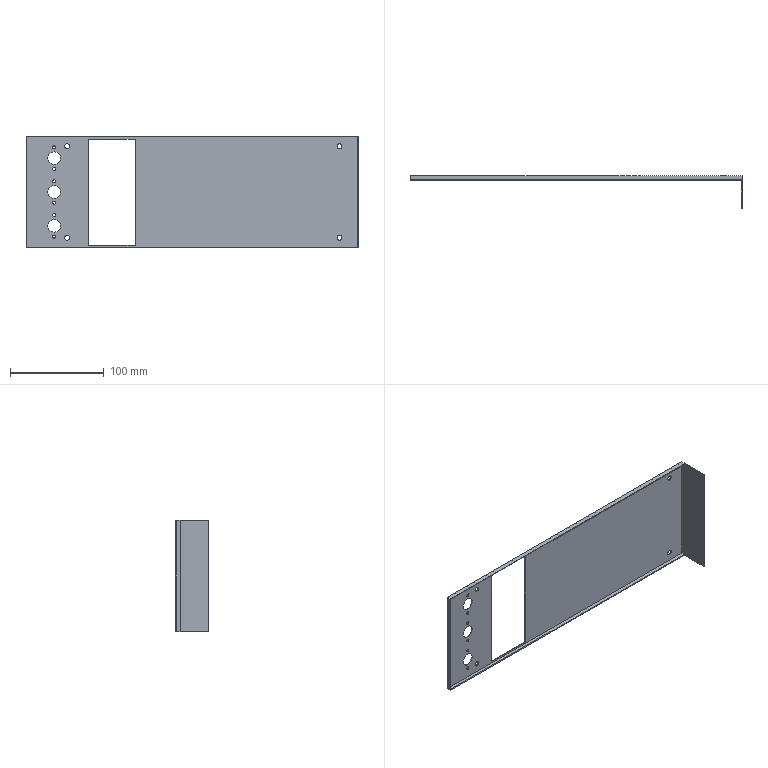Part | SolidWorks | features MoveFace 15, ICE 6, Cut 1, Extrusion 1 | 1 solid | 42 faces | box 353.4 x 34.5 x 119.15 mm | volume 42763 mm3 | cylinder 26 | plane 16 | commonest cylinder face diameters 3.2 x12 5.2 x8 13.5 x6
STEP:
#1=CARTESIAN_POINT('',(-211.2,0.5,49.1));
#2=VERTEX_POINT('',#1);
#3=CARTESIAN_POINT('',(-211.2,0.5,45.9));
#4=VERTEX_POINT('',#3);
#5=CARTESIAN_POINT('',(-211.2,0.5,47.5));
#6=DIRECTION('',(0.,-1.,0.));
#7=DIRECTION('',(0.,0.,-1.));
#8=AXIS2_PLACEMENT_3D('',#5,#6,#7);
#9=CIRCLE('',#8,1.6);
#10=EDGE_CURVE('',#2,#4,#9,.T.);
#11=ORIENTED_EDGE('',*,*,#10,.T.);
#12=CARTESIAN_POINT('',(-211.2,1.5,45.9));
#13=VERTEX_POINT('',#12);
#14=CARTESIAN_POINT('',(-211.2,-3.,45.9));
#15=DIRECTION('',(0.,1.,0.));
#16=VECTOR('',#15,1000.);
#17=LINE('',#14,#16);
#18=EDGE_CURVE('',#4,#13,#17,.T.);
#19=ORIENTED_EDGE('',*,*,#18,.T.);
#20=CARTESIAN_POINT('',(-211.2,1.5,49.1));
#21=VERTEX_POINT('',#20);
#22=CARTESIAN_POINT('',(-211.2,1.5,47.5));
#23=DIRECTION('',(0.,1.,0.));
#24=DIRECTION('',(0.,0.,1.));
#25=AXIS2_PLACEMENT_3D('',#22,#23,#24);
#26=CIRCLE('',#25,1.6);
#27=EDGE_CURVE('',#13,#21,#26,.T.);
#28=ORIENTED_EDGE('',*,*,#27,.T.);
#29=CARTESIAN_POINT('',(-211.2,-3.,49.1));
#30=DIRECTION('',(0.,1.,0.));
#31=VECTOR('',#30,1000.);
#32=LINE('',#29,#31);
#33=EDGE_CURVE('',#2,#21,#32,.T.);
#34=ORIENTED_EDGE('',*,*,#33,.F.);
#35=EDGE_LOOP('',(#11,#19,#28,#34));
#36=FACE_OUTER_BOUND('',#35,.T.);
#37=CARTESIAN_POINT('',(-211.2,-3.,47.5));
#38=DIRECTION('',(0.,1.,0.));
#39=DIRECTION('',(0.,0.,1.));
#40=AXIS2_PLACEMENT_3D('',#37,#38,#39);
#41=CYLINDRICAL_SURFACE('',#40,1.6);
#42=ADVANCED_FACE('',(#36),#41,.F.);
#43=CARTESIAN_POINT('',(-211.2,0.5,26.1));
#44=VERTEX_POINT('',#43);
#45=CARTESIAN_POINT('',(-211.2,0.5,22.9));
#46=VERTEX_POINT('',#45);
#47=CARTESIAN_POINT('',(-211.2,0.5,24.5));
#48=DIRECTION('',(0.,-1.,0.));
#49=DIRECTION('',(0.,0.,-1.));
#50=AXIS2_PLACEMENT_3D('',#47,#48,#49);
#51=CIRCLE('',#50,1.6);
#52=EDGE_CURVE('',#44,#46,#51,.T.);
#53=ORIENTED_EDGE('',*,*,#52,.T.);
#54=CARTESIAN_POINT('',(-211.2,1.5,22.9));
#55=VERTEX_POINT('',#54);
#56=CARTESIAN_POINT('',(-211.2,-3.,22.9));
#57=DIRECTION('',(0.,1.,0.));
#58=VECTOR('',#57,1000.);
#59=LINE('',#56,#58);
#60=EDGE_CURVE('',#46,#55,#59,.T.);
#61=ORIENTED_EDGE('',*,*,#60,.T.);
#62=CARTESIAN_POINT('',(-211.2,1.5,26.1));
#63=VERTEX_POINT('',#62);
#64=CARTESIAN_POINT('',(-211.2,1.5,24.5));
#65=DIRECTION('',(0.,1.,0.));
#66=DIRECTION('',(0.,0.,1.));
#67=AXIS2_PLACEMENT_3D('',#64,#65,#66);
#68=CIRCLE('',#67,1.6);
#69=EDGE_CURVE('',#55,#63,#68,.T.);
#70=ORIENTED_EDGE('',*,*,#69,.T.);
#71=CARTESIAN_POINT('',(-211.2,-3.,26.1));
#72=DIRECTION('',(0.,1.,0.));
#73=VECTOR('',#72,1000.);
#74=LINE('',#71,#73);
#75=EDGE_CURVE('',#44,#63,#74,.T.);
#76=ORIENTED_EDGE('',*,*,#75,.F.);
#77=EDGE_LOOP('',(#53,#61,#70,#76));
#78=FACE_OUTER_BOUND('',#77,.T.);
#79=CARTESIAN_POINT('',(-211.2,-3.,24.5));
#80=DIRECTION('',(0.,1.,0.));
#81=DIRECTION('',(0.,0.,1.));
#82=AXIS2_PLACEMENT_3D('',#79,#80,#81);
#83=CYLINDRICAL_SURFACE('',#82,1.6);
#84=ADVANCED_FACE('',(#78),#83,.F.);
#85=CARTESIAN_POINT('',(-211.2,0.5,13.1));
#86=VERTEX_POINT('',#85);
#87=CARTESIAN_POINT('',(-211.2,0.5,9.9));
#88=VERTEX_POINT('',#87);
#89=CARTESIAN_POINT('',(-211.2,0.5,11.5));
#90=DIRECTION('',(0.,-1.,0.));
#91=DIRECTION('',(0.,0.,-1.));
#92=AXIS2_PLACEMENT_3D('',#89,#90,#91);
#93=CIRCLE('',#92,1.6);
#94=EDGE_CURVE('',#86,#88,#93,.T.);
#95=ORIENTED_EDGE('',*,*,#94,.T.);
#96=CARTESIAN_POINT('',(-211.2,1.5,9.9));
#97=VERTEX_POINT('',#96);
#98=CARTESIAN_POINT('',(-211.2,-3.,9.9));
#99=DIRECTION('',(0.,1.,0.));
#100=VECTOR('',#99,1000.);
#101=LINE('',#98,#100);
#102=EDGE_CURVE('',#88,#97,#101,.T.);
#103=ORIENTED_EDGE('',*,*,#102,.T.);
#104=CARTESIAN_POINT('',(-211.2,1.5,13.1));
#105=VERTEX_POINT('',#104);
#106=CARTESIAN_POINT('',(-211.2,1.5,11.5));
#107=DIRECTION('',(0.,1.,0.));
#108=DIRECTION('',(0.,0.,1.));
#109=AXIS2_PLACEMENT_3D('',#106,#107,#108);
#110=CIRCLE('',#109,1.6);
#111=EDGE_CURVE('',#97,#105,#110,.T.);
#112=ORIENTED_EDGE('',*,*,#111,.T.);
#113=CARTESIAN_POINT('',(-211.2,-3.,13.1));
#114=DIRECTION('',(0.,1.,0.));
#115=VECTOR('',#114,1000.);
#116=LINE('',#113,#115);
#117=EDGE_CURVE('',#86,#105,#116,.T.);
#118=ORIENTED_EDGE('',*,*,#117,.F.);
#119=EDGE_LOOP('',(#95,#103,#112,#118));
#120=FACE_OUTER_BOUND('',#119,.T.);
#121=CARTESIAN_POINT('',(-211.2,-3.,11.5));
#122=DIRECTION('',(0.,1.,0.));
#123=DIRECTION('',(0.,0.,1.));
#124=AXIS2_PLACEMENT_3D('',#121,#122,#123);
#125=CYLINDRICAL_SURFACE('',#124,1.6);
#126=ADVANCED_FACE('',(#120),#125,.F.);
#127=CARTESIAN_POINT('',(-211.2,0.5,-9.9));
#128=VERTEX_POINT('',#127);
#129=CARTESIAN_POINT('',(-211.2,0.5,-13.1));
#130=VERTEX_POINT('',#129);
#131=CARTESIAN_POINT('',(-211.2,0.5,-11.5));
#132=DIRECTION('',(0.,-1.,0.));
#133=DIRECTION('',(0.,0.,-1.));
#134=AXIS2_PLACEMENT_3D('',#131,#132,#133);
#135=CIRCLE('',#134,1.6);
#136=EDGE_CURVE('',#128,#130,#135,.T.);
#137=ORIENTED_EDGE('',*,*,#136,.T.);
#138=CARTESIAN_POINT('',(-211.2,1.5,-13.1));
#139=VERTEX_POINT('',#138);
#140=CARTESIAN_POINT('',(-211.2,-3.,-13.1));
#141=DIRECTION('',(0.,1.,0.));
#142=VECTOR('',#141,1000.);
#143=LINE('',#140,#142);
#144=EDGE_CURVE('',#130,#139,#143,.T.);
#145=ORIENTED_EDGE('',*,*,#144,.T.);
#146=CARTESIAN_POINT('',(-211.2,1.5,-9.9));
#147=VERTEX_POINT('',#146);
#148=CARTESIAN_POINT('',(-211.2,1.5,-11.5));
#149=DIRECTION('',(0.,1.,0.));
#150=DIRECTION('',(0.,0.,1.));
#151=AXIS2_PLACEMENT_3D('',#148,#149,#150);
#152=CIRCLE('',#151,1.6);
#153=EDGE_CURVE('',#139,#147,#152,.T.);
#154=ORIENTED_EDGE('',*,*,#153,.T.);
#155=CARTESIAN_POINT('',(-211.2,-3.,-9.9));
#156=DIRECTION('',(0.,1.,0.));
#157=VECTOR('',#156,1000.);
#158=LINE('',#155,#157);
#159=EDGE_CURVE('',#128,#147,#158,.T.);
#160=ORIENTED_EDGE('',*,*,#159,.F.);
#161=EDGE_LOOP('',(#137,#145,#154,#160));
#162=FACE_OUTER_BOUND('',#161,.T.);
#163=CARTESIAN_POINT('',(-211.2,-3.,-11.5));
#164=DIRECTION('',(0.,1.,0.));
#165=DIRECTION('',(0.,0.,1.));
#166=AXIS2_PLACEMENT_3D('',#163,#164,#165);
#167=CYLINDRICAL_SURFACE('',#166,1.6);
#168=ADVANCED_FACE('',(#162),#167,.F.);
#169=CARTESIAN_POINT('',(-211.2,0.5,-22.9));
#170=VERTEX_POINT('',#169);
#171=CARTESIAN_POINT('',(-211.2,0.5,-26.1));
#172=VERTEX_POINT('',#171);
#173=CARTESIAN_POINT('',(-211.2,0.5,-24.5));
#174=DIRECTION('',(0.,-1.,0.));
#175=DIRECTION('',(0.,0.,-1.));
#176=AXIS2_PLACEMENT_3D('',#173,#174,#175);
#177=CIRCLE('',#176,1.6);
#178=EDGE_CURVE('',#170,#172,#177,.T.);
#179=ORIENTED_EDGE('',*,*,#178,.T.);
#180=CARTESIAN_POINT('',(-211.2,1.5,-26.1));
#181=VERTEX_POINT('',#180);
#182=CARTESIAN_POINT('',(-211.2,-3.,-26.1));
#183=DIRECTION('',(0.,1.,0.));
#184=VECTOR('',#183,1000.);
#185=LINE('',#182,#184);
#186=EDGE_CURVE('',#172,#181,#185,.T.);
#187=ORIENTED_EDGE('',*,*,#186,.T.);
#188=CARTESIAN_POINT('',(-211.2,1.5,-22.9));
#189=VERTEX_POINT('',#188);
#190=CARTESIAN_POINT('',(-211.2,1.5,-24.5));
#191=DIRECTION('',(0.,1.,0.));
#192=DIRECTION('',(0.,0.,1.));
#193=AXIS2_PLACEMENT_3D('',#190,#191,#192);
#194=CIRCLE('',#193,1.6);
#195=EDGE_CURVE('',#181,#189,#194,.T.);
#196=ORIENTED_EDGE('',*,*,#195,.T.);
#197=CARTESIAN_POINT('',(-211.2,-3.,-22.9));
#198=DIRECTION('',(0.,1.,0.));
#199=VECTOR('',#198,1000.);
#200=LINE('',#197,#199);
#201=EDGE_CURVE('',#170,#189,#200,.T.);
#202=ORIENTED_EDGE('',*,*,#201,.F.);
#203=EDGE_LOOP('',(#179,#187,#196,#202));
#204=FACE_OUTER_BOUND('',#203,.T.);
#205=CARTESIAN_POINT('',(-211.2,-3.,-24.5));
#206=DIRECTION('',(0.,1.,0.));
#207=DIRECTION('',(0.,0.,1.));
#208=AXIS2_PLACEMENT_3D('',#205,#206,#207);
#209=CYLINDRICAL_SURFACE('',#208,1.6);
#210=ADVANCED_FACE('',(#204),#209,.F.);
#211=CARTESIAN_POINT('',(-211.2,0.5,-45.9));
#212=VERTEX_POINT('',#211);
#213=CARTESIAN_POINT('',(-211.2,0.5,-49.1));
#214=VERTEX_POINT('',#213);
#215=CARTESIAN_POINT('',(-211.2,0.5,-47.5));
#216=DIRECTION('',(0.,-1.,0.));
#217=DIRECTION('',(0.,0.,-1.));
#218=AXIS2_PLACEMENT_3D('',#215,#216,#217);
#219=CIRCLE('',#218,1.6);
#220=EDGE_CURVE('',#212,#214,#219,.T.);
#221=ORIENTED_EDGE('',*,*,#220,.T.);
#222=CARTESIAN_POINT('',(-211.2,1.5,-49.1));
#223=VERTEX_POINT('',#222);
#224=CARTESIAN_POINT('',(-211.2,-3.,-49.1));
#225=DIRECTION('',(0.,1.,0.));
#226=VECTOR('',#225,1000.);
#227=LINE('',#224,#226);
#228=EDGE_CURVE('',#214,#223,#227,.T.);
#229=ORIENTED_EDGE('',*,*,#228,.T.);
#230=CARTESIAN_POINT('',(-211.2,1.5,-45.9));
#231=VERTEX_POINT('',#230);
#232=CARTESIAN_POINT('',(-211.2,1.5,-47.5));
#233=DIRECTION('',(0.,1.,0.));
#234=DIRECTION('',(0.,0.,1.));
#235=AXIS2_PLACEMENT_3D('',#232,#233,#234);
#236=CIRCLE('',#235,1.6);
#237=EDGE_CURVE('',#223,#231,#236,.T.);
#238=ORIENTED_EDGE('',*,*,#237,.T.);
#239=CARTESIAN_POINT('',(-211.2,-3.,-45.9));
#240=DIRECTION('',(0.,1.,0.));
#241=VECTOR('',#240,1000.);
#242=LINE('',#239,#241);
#243=EDGE_CURVE('',#212,#231,#242,.T.);
#244=ORIENTED_EDGE('',*,*,#243,.F.);
#245=EDGE_LOOP('',(#221,#229,#238,#244));
#246=FACE_OUTER_BOUND('',#245,.T.);
#247=CARTESIAN_POINT('',(-211.2,-3.,-47.5));
#248=DIRECTION('',(0.,1.,0.));
#249=DIRECTION('',(0.,0.,1.));
#250=AXIS2_PLACEMENT_3D('',#247,#248,#249);
#251=CYLINDRICAL_SURFACE('',#250,1.6);
#252=ADVANCED_FACE('',(#246),#251,.F.);
#253=CARTESIAN_POINT('',(-211.2,0.5,42.75));
#254=VERTEX_POINT('',#253);
#255=CARTESIAN_POINT('',(-211.2,0.5,29.25));
#256=VERTEX_POINT('',#255);
#257=CARTESIAN_POINT('',(-211.2,0.5,36.));
#258=DIRECTION('',(0.,-1.,0.));
#259=DIRECTION('',(0.,0.,-1.));
#260=AXIS2_PLACEMENT_3D('',#257,#258,#259);
#261=CIRCLE('',#260,6.75);
#262=EDGE_CURVE('',#254,#256,#261,.T.);
#263=ORIENTED_EDGE('',*,*,#262,.T.);
#264=CARTESIAN_POINT('',(-211.2,1.5,29.25));
#265=VERTEX_POINT('',#264);
#266=CARTESIAN_POINT('',(-211.2,-8.5,29.25));
#267=DIRECTION('',(0.,1.,0.));
#268=VECTOR('',#267,1000.);
#269=LINE('',#266,#268);
#270=EDGE_CURVE('',#256,#265,#269,.T.);
#271=ORIENTED_EDGE('',*,*,#270,.T.);
#272=CARTESIAN_POINT('',(-211.2,1.5,42.75));
#273=VERTEX_POINT('',#272);
#274=CARTESIAN_POINT('',(-211.2,1.5,36.));
#275=DIRECTION('',(0.,1.,0.));
#276=DIRECTION('',(0.,0.,1.));
#277=AXIS2_PLACEMENT_3D('',#274,#275,#276);
#278=CIRCLE('',#277,6.75);
#279=EDGE_CURVE('',#265,#273,#278,.T.);
#280=ORIENTED_EDGE('',*,*,#279,.T.);
#281=CARTESIAN_POINT('',(-211.2,-8.5,42.75));
#282=DIRECTION('',(0.,1.,0.));
#283=VECTOR('',#282,1000.);
#284=LINE('',#281,#283);
#285=EDGE_CURVE('',#254,#273,#284,.T.);
#286=ORIENTED_EDGE('',*,*,#285,.F.);
#287=EDGE_LOOP('',(#263,#271,#280,#286));
#288=FACE_OUTER_BOUND('',#287,.T.);
#289=CARTESIAN_POINT('',(-211.2,-8.5,36.));
#290=DIRECTION('',(0.,1.,0.));
#291=DIRECTION('',(0.,0.,1.));
#292=AXIS2_PLACEMENT_3D('',#289,#290,#291);
#293=CYLINDRICAL_SURFACE('',#292,6.75);
#294=ADVANCED_FACE('',(#288),#293,.F.);
#295=CARTESIAN_POINT('',(-211.2,0.5,6.75));
#296=VERTEX_POINT('',#295);
#297=CARTESIAN_POINT('',(-211.2,0.5,-6.75));
#298=VERTEX_POINT('',#297);
#299=CARTESIAN_POINT('',(-211.2,0.5,0.));
#300=DIRECTION('',(0.,-1.,0.));
#301=DIRECTION('',(0.,0.,-1.));
#302=AXIS2_PLACEMENT_3D('',#299,#300,#301);
#303=CIRCLE('',#302,6.75);
#304=EDGE_CURVE('',#296,#298,#303,.T.);
#305=ORIENTED_EDGE('',*,*,#304,.T.);
#306=CARTESIAN_POINT('',(-211.2,1.5,-6.75));
#307=VERTEX_POINT('',#306);
#308=CARTESIAN_POINT('',(-211.2,-8.5,-6.75));
#309=DIRECTION('',(0.,1.,0.));
#310=VECTOR('',#309,1000.);
#311=LINE('',#308,#310);
#312=EDGE_CURVE('',#298,#307,#311,.T.);
#313=ORIENTED_EDGE('',*,*,#312,.T.);
#314=CARTESIAN_POINT('',(-211.2,1.5,6.75));
#315=VERTEX_POINT('',#314);
#316=CARTESIAN_POINT('',(-211.2,1.5,0.));
#317=DIRECTION('',(0.,1.,0.));
#318=DIRECTION('',(0.,0.,1.));
#319=AXIS2_PLACEMENT_3D('',#316,#317,#318);
#320=CIRCLE('',#319,6.75);
#321=EDGE_CURVE('',#307,#315,#320,.T.);
#322=ORIENTED_EDGE('',*,*,#321,.T.);
#323=CARTESIAN_POINT('',(-211.2,-8.5,6.75));
#324=DIRECTION('',(0.,1.,0.));
#325=VECTOR('',#324,1000.);
#326=LINE('',#323,#325);
#327=EDGE_CURVE('',#296,#315,#326,.T.);
#328=ORIENTED_EDGE('',*,*,#327,.F.);
#329=EDGE_LOOP('',(#305,#313,#322,#328));
#330=FACE_OUTER_BOUND('',#329,.T.);
#331=CARTESIAN_POINT('',(-211.2,-8.5,0.));
#332=DIRECTION('',(0.,1.,0.));
#333=DIRECTION('',(0.,0.,1.));
#334=AXIS2_PLACEMENT_3D('',#331,#332,#333);
#335=CYLINDRICAL_SURFACE('',#334,6.75);
#336=ADVANCED_FACE('',(#330),#335,.F.);
#337=CARTESIAN_POINT('',(-211.2,0.5,-29.25));
#338=VERTEX_POINT('',#337);
#339=CARTESIAN_POINT('',(-211.2,0.5,-42.75));
#340=VERTEX_POINT('',#339);
#341=CARTESIAN_POINT('',(-211.2,0.5,-36.));
#342=DIRECTION('',(0.,-1.,0.));
#343=DIRECTION('',(0.,0.,-1.));
#344=AXIS2_PLACEMENT_3D('',#341,#342,#343);
#345=CIRCLE('',#344,6.75);
#346=EDGE_CURVE('',#338,#340,#345,.T.);
#347=ORIENTED_EDGE('',*,*,#346,.T.);
#348=CARTESIAN_POINT('',(-211.2,1.5,-42.75));
#349=VERTEX_POINT('',#348);
#350=CARTESIAN_POINT('',(-211.2,-8.5,-42.75));
#351=DIRECTION('',(0.,1.,0.));
#352=VECTOR('',#351,1000.);
#353=LINE('',#350,#352);
#354=EDGE_CURVE('',#340,#349,#353,.T.);
#355=ORIENTED_EDGE('',*,*,#354,.T.);
#356=CARTESIAN_POINT('',(-211.2,1.5,-29.25));
#357=VERTEX_POINT('',#356);
#358=CARTESIAN_POINT('',(-211.2,1.5,-36.));
#359=DIRECTION('',(0.,1.,0.));
#360=DIRECTION('',(0.,0.,1.));
#361=AXIS2_PLACEMENT_3D('',#358,#359,#360);
#362=CIRCLE('',#361,6.75);
#363=EDGE_CURVE('',#349,#357,#362,.T.);
#364=ORIENTED_EDGE('',*,*,#363,.T.);
#365=CARTESIAN_POINT('',(-211.2,-8.5,-29.25));
#366=DIRECTION('',(0.,1.,0.));
#367=VECTOR('',#366,1000.);
#368=LINE('',#365,#367);
#369=EDGE_CURVE('',#338,#357,#368,.T.);
#370=ORIENTED_EDGE('',*,*,#369,.F.);
#371=EDGE_LOOP('',(#347,#355,#364,#370));
#372=FACE_OUTER_BOUND('',#371,.T.);
#373=CARTESIAN_POINT('',(-211.2,-8.5,-36.));
#374=DIRECTION('',(0.,1.,0.));
#375=DIRECTION('',(0.,0.,1.));
#376=AXIS2_PLACEMENT_3D('',#373,#374,#375);
#377=CYLINDRICAL_SURFACE('',#376,6.75);
#378=ADVANCED_FACE('',(#372),#377,.F.);
#379=CARTESIAN_POINT('',(92.5,0.5,-46.025));
#380=VERTEX_POINT('',#379);
#381=CARTESIAN_POINT('',(92.5,0.5,-51.225));
#382=VERTEX_POINT('',#381);
#383=CARTESIAN_POINT('',(92.5,0.5,-48.625));
#384=DIRECTION('',(0.,-1.,0.));
#385=DIRECTION('',(0.,0.,-1.));
#386=AXIS2_PLACEMENT_3D('',#383,#384,#385);
#387=CIRCLE('',#386,2.6);
#388=EDGE_CURVE('',#380,#382,#387,.T.);
#389=ORIENTED_EDGE('',*,*,#388,.T.);
#390=CARTESIAN_POINT('',(92.5,1.5,-51.225));
#391=VERTEX_POINT('',#390);
#392=CARTESIAN_POINT('',(92.5,-330.5,-51.225));
#393=DIRECTION('',(0.,1.,0.));
#394=VECTOR('',#393,1000.);
#395=LINE('',#392,#394);
#396=EDGE_CURVE('',#382,#391,#395,.T.);
#397=ORIENTED_EDGE('',*,*,#396,.T.);
#398=CARTESIAN_POINT('',(92.5,1.5,-46.025));
#399=VERTEX_POINT('',#398);
#400=CARTESIAN_POINT('',(92.5,1.5,-48.625));
#401=DIRECTION('',(0.,1.,0.));
#402=DIRECTION('',(0.,0.,1.));
#403=AXIS2_PLACEMENT_3D('',#400,#401,#402);
#404=CIRCLE('',#403,2.6);
#405=EDGE_CURVE('',#391,#399,#404,.T.);
#406=ORIENTED_EDGE('',*,*,#405,.T.);
#407=CARTESIAN_POINT('',(92.5,-330.5,-46.025));
#408=DIRECTION('',(0.,1.,0.));
#409=VECTOR('',#408,1000.);
#410=LINE('',#407,#409);
#411=EDGE_CURVE('',#380,#399,#410,.T.);
#412=ORIENTED_EDGE('',*,*,#411,.F.);
#413=EDGE_LOOP('',(#389,#397,#406,#412));
#414=FACE_OUTER_BOUND('',#413,.T.);
#415=CARTESIAN_POINT('',(92.5,-330.5,-48.625));
#416=DIRECTION('',(0.,1.,0.));
#417=DIRECTION('',(0.,0.,1.));
#418=AXIS2_PLACEMENT_3D('',#415,#416,#417);
#419=CYLINDRICAL_SURFACE('',#418,2.6);
#420=ADVANCED_FACE('',(#414),#419,.F.);
#421=CARTESIAN_POINT('',(-197.5,0.5,51.225));
#422=VERTEX_POINT('',#421);
#423=CARTESIAN_POINT('',(-197.5,0.5,46.025));
#424=VERTEX_POINT('',#423);
#425=CARTESIAN_POINT('',(-197.5,0.5,48.625));
#426=DIRECTION('',(0.,-1.,0.));
#427=DIRECTION('',(0.,0.,-1.));
#428=AXIS2_PLACEMENT_3D('',#425,#426,#427);
#429=CIRCLE('',#428,2.6);
#430=EDGE_CURVE('',#422,#424,#429,.T.);
#431=ORIENTED_EDGE('',*,*,#430,.T.);
#432=CARTESIAN_POINT('',(-197.5,1.5,46.025));
#433=VERTEX_POINT('',#432);
#434=CARTESIAN_POINT('',(-197.5,-330.5,46.025));
#435=DIRECTION('',(0.,1.,0.));
#436=VECTOR('',#435,1000.);
#437=LINE('',#434,#436);
#438=EDGE_CURVE('',#424,#433,#437,.T.);
#439=ORIENTED_EDGE('',*,*,#438,.T.);
#440=CARTESIAN_POINT('',(-197.5,1.5,51.225));
#441=VERTEX_POINT('',#440);
#442=CARTESIAN_POINT('',(-197.5,1.5,48.625));
#443=DIRECTION('',(0.,1.,0.));
#444=DIRECTION('',(0.,0.,1.));
#445=AXIS2_PLACEMENT_3D('',#442,#443,#444);
#446=CIRCLE('',#445,2.6);
#447=EDGE_CURVE('',#433,#441,#446,.T.);
#448=ORIENTED_EDGE('',*,*,#447,.T.);
#449=CARTESIAN_POINT('',(-197.5,-330.5,51.225));
#450=DIRECTION('',(0.,1.,0.));
#451=VECTOR('',#450,1000.);
#452=LINE('',#449,#451);
#453=EDGE_CURVE('',#422,#441,#452,.T.);
#454=ORIENTED_EDGE('',*,*,#453,.F.);
#455=EDGE_LOOP('',(#431,#439,#448,#454));
#456=FACE_OUTER_BOUND('',#455,.T.);
#457=CARTESIAN_POINT('',(-197.5,-330.5,48.625));
#458=DIRECTION('',(0.,1.,0.));
#459=DIRECTION('',(0.,0.,1.));
#460=AXIS2_PLACEMENT_3D('',#457,#458,#459);
#461=CYLINDRICAL_SURFACE('',#460,2.6);
#462=ADVANCED_FACE('',(#456),#461,.F.);
#463=CARTESIAN_POINT('',(-197.5,0.5,-46.025));
#464=VERTEX_POINT('',#463);
#465=CARTESIAN_POINT('',(-197.5,0.5,-51.225));
#466=VERTEX_POINT('',#465);
#467=CARTESIAN_POINT('',(-197.5,0.5,-48.625));
#468=DIRECTION('',(0.,-1.,0.));
#469=DIRECTION('',(0.,0.,-1.));
#470=AXIS2_PLACEMENT_3D('',#467,#468,#469);
#471=CIRCLE('',#470,2.6);
#472=EDGE_CURVE('',#464,#466,#471,.T.);
#473=ORIENTED_EDGE('',*,*,#472,.T.);
#474=CARTESIAN_POINT('',(-197.5,1.5,-51.225));
#475=VERTEX_POINT('',#474);
#476=CARTESIAN_POINT('',(-197.5,-330.5,-51.225));
#477=DIRECTION('',(0.,1.,0.));
#478=VECTOR('',#477,1000.);
#479=LINE('',#476,#478);
#480=EDGE_CURVE('',#466,#475,#479,.T.);
#481=ORIENTED_EDGE('',*,*,#480,.T.);
#482=CARTESIAN_POINT('',(-197.5,1.5,-46.025));
#483=VERTEX_POINT('',#482);
#484=CARTESIAN_POINT('',(-197.5,1.5,-48.625));
#485=DIRECTION('',(0.,1.,0.));
#486=DIRECTION('',(0.,0.,1.));
#487=AXIS2_PLACEMENT_3D('',#484,#485,#486);
#488=CIRCLE('',#487,2.6);
#489=EDGE_CURVE('',#475,#483,#488,.T.);
#490=ORIENTED_EDGE('',*,*,#489,.T.);
#491=CARTESIAN_POINT('',(-197.5,-330.5,-46.025));
#492=DIRECTION('',(0.,1.,0.));
#493=VECTOR('',#492,1000.);
#494=LINE('',#491,#493);
#495=EDGE_CURVE('',#464,#483,#494,.T.);
#496=ORIENTED_EDGE('',*,*,#495,.F.);
#497=EDGE_LOOP('',(#473,#481,#490,#496));
#498=FACE_OUTER_BOUND('',#497,.T.);
#499=CARTESIAN_POINT('',(-197.5,-330.5,-48.625));
#500=DIRECTION('',(0.,1.,0.));
#501=DIRECTION('',(0.,0.,1.));
#502=AXIS2_PLACEMENT_3D('',#499,#500,#501);
#503=CYLINDRICAL_SURFACE('',#502,2.6);
#504=ADVANCED_FACE('',(#498),#503,.F.);
#505=CARTESIAN_POINT('',(92.5,0.5,51.225));
#506=VERTEX_POINT('',#505);
#507=CARTESIAN_POINT('',(92.5,0.5,46.025));
#508=VERTEX_POINT('',#507);
#509=CARTESIAN_POINT('',(92.5,0.5,48.625));
#510=DIRECTION('',(0.,-1.,0.));
#511=DIRECTION('',(0.,0.,-1.));
#512=AXIS2_PLACEMENT_3D('',#509,#510,#511);
#513=CIRCLE('',#512,2.6);
#514=EDGE_CURVE('',#506,#508,#513,.T.);
#515=ORIENTED_EDGE('',*,*,#514,.T.);
#516=CARTESIAN_POINT('',(92.5,1.5,46.025));
#517=VERTEX_POINT('',#516);
#518=CARTESIAN_POINT('',(92.5,-330.5,46.025));
#519=DIRECTION('',(0.,1.,0.));
#520=VECTOR('',#519,1000.);
#521=LINE('',#518,#520);
#522=EDGE_CURVE('',#508,#517,#521,.T.);
#523=ORIENTED_EDGE('',*,*,#522,.T.);
#524=CARTESIAN_POINT('',(92.5,1.5,51.225));
#525=VERTEX_POINT('',#524);
#526=CARTESIAN_POINT('',(92.5,1.5,48.625));
#527=DIRECTION('',(0.,1.,0.));
#528=DIRECTION('',(0.,0.,1.));
#529=AXIS2_PLACEMENT_3D('',#526,#527,#528);
#530=CIRCLE('',#529,2.6);
#531=EDGE_CURVE('',#517,#525,#530,.T.);
#532=ORIENTED_EDGE('',*,*,#531,.T.);
#533=CARTESIAN_POINT('',(92.5,-330.5,51.225));
#534=DIRECTION('',(0.,1.,0.));
#535=VECTOR('',#534,1000.);
#536=LINE('',#533,#535);
#537=EDGE_CURVE('',#506,#525,#536,.T.);
#538=ORIENTED_EDGE('',*,*,#537,.F.);
#539=EDGE_LOOP('',(#515,#523,#532,#538));
#540=FACE_OUTER_BOUND('',#539,.T.);
#541=CARTESIAN_POINT('',(92.5,-330.5,48.625));
#542=DIRECTION('',(0.,1.,0.));
#543=DIRECTION('',(0.,0.,1.));
#544=AXIS2_PLACEMENT_3D('',#541,#542,#543);
#545=CYLINDRICAL_SURFACE('',#544,2.6);
#546=ADVANCED_FACE('',(#540),#545,.F.);
#547=CARTESIAN_POINT('',(-211.2,1.5,47.5));
#548=DIRECTION('',(0.,1.,0.));
#549=DIRECTION('',(0.,0.,1.));
#550=AXIS2_PLACEMENT_3D('',#547,#548,#549);
#551=CIRCLE('',#550,1.6);
#552=EDGE_CURVE('',#21,#13,#551,.T.);
#553=ORIENTED_EDGE('',*,*,#552,.F.);
#554=ORIENTED_EDGE('',*,*,#27,.F.);
#555=EDGE_LOOP('',(#553,#554));
#556=FACE_BOUND('',#555,.T.);
#557=CARTESIAN_POINT('',(-211.2,1.5,24.5));
#558=DIRECTION('',(0.,1.,0.));
#559=DIRECTION('',(0.,0.,1.));
#560=AXIS2_PLACEMENT_3D('',#557,#558,#559);
#561=CIRCLE('',#560,1.6);
#562=EDGE_CURVE('',#63,#55,#561,.T.);
#563=ORIENTED_EDGE('',*,*,#562,.F.);
#564=ORIENTED_EDGE('',*,*,#69,.F.);
#565=EDGE_LOOP('',(#563,#564));
#566=FACE_BOUND('',#565,.T.);
#567=CARTESIAN_POINT('',(-211.2,1.5,11.5));
#568=DIRECTION('',(0.,1.,0.));
#569=DIRECTION('',(0.,0.,1.));
#570=AXIS2_PLACEMENT_3D('',#567,#568,#569);
#571=CIRCLE('',#570,1.6);
#572=EDGE_CURVE('',#105,#97,#571,.T.);
#573=ORIENTED_EDGE('',*,*,#572,.F.);
#574=ORIENTED_EDGE('',*,*,#111,.F.);
#575=EDGE_LOOP('',(#573,#574));
#576=FACE_BOUND('',#575,.T.);
#577=CARTESIAN_POINT('',(-211.2,1.5,-11.5));
#578=DIRECTION('',(0.,1.,0.));
#579=DIRECTION('',(0.,0.,1.));
#580=AXIS2_PLACEMENT_3D('',#577,#578,#579);
#581=CIRCLE('',#580,1.6);
#582=EDGE_CURVE('',#147,#139,#581,.T.);
#583=ORIENTED_EDGE('',*,*,#582,.F.);
#584=ORIENTED_EDGE('',*,*,#153,.F.);
#585=EDGE_LOOP('',(#583,#584));
#586=FACE_BOUND('',#585,.T.);
#587=CARTESIAN_POINT('',(-211.2,1.5,-24.5));
#588=DIRECTION('',(0.,1.,0.));
#589=DIRECTION('',(0.,0.,1.));
#590=AXIS2_PLACEMENT_3D('',#587,#588,#589);
#591=CIRCLE('',#590,1.6);
#592=EDGE_CURVE('',#189,#181,#591,.T.);
#593=ORIENTED_EDGE('',*,*,#592,.F.);
#594=ORIENTED_EDGE('',*,*,#195,.F.);
#595=EDGE_LOOP('',(#593,#594));
#596=FACE_BOUND('',#595,.T.);
#597=CARTESIAN_POINT('',(-211.2,1.5,-47.5));
#598=DIRECTION('',(0.,1.,0.));
#599=DIRECTION('',(0.,0.,1.));
#600=AXIS2_PLACEMENT_3D('',#597,#598,#599);
#601=CIRCLE('',#600,1.6);
#602=EDGE_CURVE('',#231,#223,#601,.T.);
#603=ORIENTED_EDGE('',*,*,#602,.F.);
#604=ORIENTED_EDGE('',*,*,#237,.F.);
#605=EDGE_LOOP('',(#603,#604));
#606=FACE_BOUND('',#605,.T.);
#607=CARTESIAN_POINT('',(-211.2,1.5,36.));
#608=DIRECTION('',(0.,1.,0.));
#609=DIRECTION('',(0.,0.,1.));
#610=AXIS2_PLACEMENT_3D('',#607,#608,#609);
#611=CIRCLE('',#610,6.75);
#612=EDGE_CURVE('',#273,#265,#611,.T.);
#613=ORIENTED_EDGE('',*,*,#612,.F.);
#614=ORIENTED_EDGE('',*,*,#279,.F.);
#615=EDGE_LOOP('',(#613,#614));
#616=FACE_BOUND('',#615,.T.);
#617=CARTESIAN_POINT('',(-211.2,1.5,0.));
#618=DIRECTION('',(0.,1.,0.));
#619=DIRECTION('',(0.,0.,1.));
#620=AXIS2_PLACEMENT_3D('',#617,#618,#619);
#621=CIRCLE('',#620,6.75);
#622=EDGE_CURVE('',#315,#307,#621,.T.);
#623=ORIENTED_EDGE('',*,*,#622,.F.);
#624=ORIENTED_EDGE('',*,*,#321,.F.);
#625=EDGE_LOOP('',(#623,#624));
#626=FACE_BOUND('',#625,.T.);
#627=CARTESIAN_POINT('',(-211.2,1.5,-36.));
#628=DIRECTION('',(0.,1.,0.));
#629=DIRECTION('',(0.,0.,1.));
#630=AXIS2_PLACEMENT_3D('',#627,#628,#629);
#631=CIRCLE('',#630,6.75);
#632=EDGE_CURVE('',#357,#349,#631,.T.);
#633=ORIENTED_EDGE('',*,*,#632,.F.);
#634=ORIENTED_EDGE('',*,*,#363,.F.);
#635=EDGE_LOOP('',(#633,#634));
#636=FACE_BOUND('',#635,.T.);
#637=CARTESIAN_POINT('',(-175.,1.5,56.075));
#638=VERTEX_POINT('',#637);
#639=CARTESIAN_POINT('',(-125.,1.5,56.075));
#640=VERTEX_POINT('',#639);
#641=CARTESIAN_POINT('',(-175.,1.5,56.075));
#642=DIRECTION('',(1.,0.,0.));
#643=VECTOR('',#642,1000.);
#644=LINE('',#641,#643);
#645=EDGE_CURVE('',#638,#640,#644,.T.);
#646=ORIENTED_EDGE('',*,*,#645,.F.);
#647=CARTESIAN_POINT('',(-175.,1.5,-56.925));
#648=VERTEX_POINT('',#647);
#649=CARTESIAN_POINT('',(-175.,1.5,57.375));
#650=DIRECTION('',(0.,0.,1.));
#651=VECTOR('',#650,1000.);
#652=LINE('',#649,#651);
#653=EDGE_CURVE('',#648,#638,#652,.T.);
#654=ORIENTED_EDGE('',*,*,#653,.F.);
#655=CARTESIAN_POINT('',(-125.,1.5,-56.925));
#656=VERTEX_POINT('',#655);
#657=CARTESIAN_POINT('',(-175.,1.5,-56.925));
#658=DIRECTION('',(-1.,0.,0.));
#659=VECTOR('',#658,1000.);
#660=LINE('',#657,#659);
#661=EDGE_CURVE('',#656,#648,#660,.T.);
#662=ORIENTED_EDGE('',*,*,#661,.F.);
#663=CARTESIAN_POINT('',(-125.,1.5,57.375));
#664=DIRECTION('',(0.,0.,-1.));
#665=VECTOR('',#664,1000.);
#666=LINE('',#663,#665);
#667=EDGE_CURVE('',#640,#656,#666,.T.);
#668=ORIENTED_EDGE('',*,*,#667,.F.);
#669=EDGE_LOOP('',(#646,#654,#662,#668));
#670=FACE_BOUND('',#669,.T.);
#671=CARTESIAN_POINT('',(92.5,1.5,-48.625));
#672=DIRECTION('',(0.,1.,0.));
#673=DIRECTION('',(0.,0.,1.));
#674=AXIS2_PLACEMENT_3D('',#671,#672,#673);
#675=CIRCLE('',#674,2.6);
#676=EDGE_CURVE('',#399,#391,#675,.T.);
#677=ORIENTED_EDGE('',*,*,#676,.F.);
#678=ORIENTED_EDGE('',*,*,#405,.F.);
#679=EDGE_LOOP('',(#677,#678));
#680=FACE_BOUND('',#679,.T.);
#681=CARTESIAN_POINT('',(-197.5,1.5,48.625));
#682=DIRECTION('',(0.,1.,0.));
#683=DIRECTION('',(0.,0.,1.));
#684=AXIS2_PLACEMENT_3D('',#681,#682,#683);
#685=CIRCLE('',#684,2.6);
#686=EDGE_CURVE('',#441,#433,#685,.T.);
#687=ORIENTED_EDGE('',*,*,#686,.F.);
#688=ORIENTED_EDGE('',*,*,#447,.F.);
#689=EDGE_LOOP('',(#687,#688));
#690=FACE_BOUND('',#689,.T.);
#691=CARTESIAN_POINT('',(-197.5,1.5,-48.625));
#692=DIRECTION('',(0.,1.,0.));
#693=DIRECTION('',(0.,0.,1.));
#694=AXIS2_PLACEMENT_3D('',#691,#692,#693);
#695=CIRCLE('',#694,2.6);
#696=EDGE_CURVE('',#483,#475,#695,.T.);
#697=ORIENTED_EDGE('',*,*,#696,.F.);
#698=ORIENTED_EDGE('',*,*,#489,.F.);
#699=EDGE_LOOP('',(#697,#698));
#700=FACE_BOUND('',#699,.T.);
#701=CARTESIAN_POINT('',(92.5,1.5,48.625));
#702=DIRECTION('',(0.,1.,0.));
#703=DIRECTION('',(0.,0.,1.));
#704=AXIS2_PLACEMENT_3D('',#701,#702,#703);
#705=CIRCLE('',#704,2.6);
#706=EDGE_CURVE('',#525,#517,#705,.T.);
#707=ORIENTED_EDGE('',*,*,#706,.F.);
#708=ORIENTED_EDGE('',*,*,#531,.F.);
#709=EDGE_LOOP('',(#707,#708));
#710=FACE_BOUND('',#709,.T.);
#711=CARTESIAN_POINT('',(-241.2,1.5,59.575));
#712=VERTEX_POINT('',#711);
#713=CARTESIAN_POINT('',(-241.2,1.5,-59.575));
#714=VERTEX_POINT('',#713);
#715=CARTESIAN_POINT('',(-241.2,1.5,-73.575));
#716=DIRECTION('',(0.,0.,-1.));
#717=VECTOR('',#716,1000.);
#718=LINE('',#715,#717);
#719=EDGE_CURVE('',#712,#714,#718,.T.);
#720=ORIENTED_EDGE('',*,*,#719,.F.);
#721=CARTESIAN_POINT('',(112.2,1.5,59.575));
#722=VERTEX_POINT('',#721);
#723=CARTESIAN_POINT('',(-241.2,1.5,59.575));
#724=DIRECTION('',(-1.,0.,0.));
#725=VECTOR('',#724,1000.);
#726=LINE('',#723,#725);
#727=EDGE_CURVE('',#722,#712,#726,.T.);
#728=ORIENTED_EDGE('',*,*,#727,.F.);
#729=CARTESIAN_POINT('',(112.2,1.5,-59.575));
#730=VERTEX_POINT('',#729);
#731=CARTESIAN_POINT('',(112.2,1.5,73.575));
#732=DIRECTION('',(0.,0.,1.));
#733=VECTOR('',#732,1000.);
#734=LINE('',#731,#733);
#735=EDGE_CURVE('',#730,#722,#734,.T.);
#736=ORIENTED_EDGE('',*,*,#735,.F.);
#737=CARTESIAN_POINT('',(151.2,1.5,-59.575));
#738=DIRECTION('',(1.,0.,0.));
#739=VECTOR('',#738,1000.);
#740=LINE('',#737,#739);
#741=EDGE_CURVE('',#714,#730,#740,.T.);
#742=ORIENTED_EDGE('',*,*,#741,.F.);
#743=EDGE_LOOP('',(#720,#728,#736,#742));
#744=FACE_OUTER_BOUND('',#743,.T.);
#745=CARTESIAN_POINT('',(0.,1.5,0.));
#746=DIRECTION('',(0.,-1.,0.));
#747=DIRECTION('',(0.,0.,-1.));
#748=AXIS2_PLACEMENT_3D('',#745,#746,#747);
#749=PLANE('',#748);
#750=ADVANCED_FACE('',(#556,#566,#576,#586,#596,#606,#616,#626,#636,#670,#680,#690,#700,#710,#744),#749,.F.);
#751=ORIENTED_EDGE('',*,*,#10,.F.);
#752=CARTESIAN_POINT('',(-211.2,0.5,47.5));
#753=DIRECTION('',(0.,-1.,0.));
#754=DIRECTION('',(0.,0.,-1.));
#755=AXIS2_PLACEMENT_3D('',#752,#753,#754);
#756=CIRCLE('',#755,1.6);
#757=EDGE_CURVE('',#4,#2,#756,.T.);
#758=ORIENTED_EDGE('',*,*,#757,.F.);
#759=EDGE_LOOP('',(#751,#758));
#760=FACE_BOUND('',#759,.T.);
#761=ORIENTED_EDGE('',*,*,#52,.F.);
#762=CARTESIAN_POINT('',(-211.2,0.5,24.5));
#763=DIRECTION('',(0.,-1.,0.));
#764=DIRECTION('',(0.,0.,-1.));
#765=AXIS2_PLACEMENT_3D('',#762,#763,#764);
#766=CIRCLE('',#765,1.6);
#767=EDGE_CURVE('',#46,#44,#766,.T.);
#768=ORIENTED_EDGE('',*,*,#767,.F.);
#769=EDGE_LOOP('',(#761,#768));
#770=FACE_BOUND('',#769,.T.);
#771=ORIENTED_EDGE('',*,*,#94,.F.);
#772=CARTESIAN_POINT('',(-211.2,0.5,11.5));
#773=DIRECTION('',(0.,-1.,0.));
#774=DIRECTION('',(0.,0.,-1.));
#775=AXIS2_PLACEMENT_3D('',#772,#773,#774);
#776=CIRCLE('',#775,1.6);
#777=EDGE_CURVE('',#88,#86,#776,.T.);
#778=ORIENTED_EDGE('',*,*,#777,.F.);
#779=EDGE_LOOP('',(#771,#778));
#780=FACE_BOUND('',#779,.T.);
#781=ORIENTED_EDGE('',*,*,#136,.F.);
#782=CARTESIAN_POINT('',(-211.2,0.5,-11.5));
#783=DIRECTION('',(0.,-1.,0.));
#784=DIRECTION('',(0.,0.,-1.));
#785=AXIS2_PLACEMENT_3D('',#782,#783,#784);
#786=CIRCLE('',#785,1.6);
#787=EDGE_CURVE('',#130,#128,#786,.T.);
#788=ORIENTED_EDGE('',*,*,#787,.F.);
#789=EDGE_LOOP('',(#781,#788));
#790=FACE_BOUND('',#789,.T.);
#791=ORIENTED_EDGE('',*,*,#178,.F.);
#792=CARTESIAN_POINT('',(-211.2,0.5,-24.5));
#793=DIRECTION('',(0.,-1.,0.));
#794=DIRECTION('',(0.,0.,-1.));
#795=AXIS2_PLACEMENT_3D('',#792,#793,#794);
#796=CIRCLE('',#795,1.6);
#797=EDGE_CURVE('',#172,#170,#796,.T.);
#798=ORIENTED_EDGE('',*,*,#797,.F.);
#799=EDGE_LOOP('',(#791,#798));
#800=FACE_BOUND('',#799,.T.);
#801=ORIENTED_EDGE('',*,*,#220,.F.);
#802=CARTESIAN_POINT('',(-211.2,0.5,-47.5));
#803=DIRECTION('',(0.,-1.,0.));
#804=DIRECTION('',(0.,0.,-1.));
#805=AXIS2_PLACEMENT_3D('',#802,#803,#804);
#806=CIRCLE('',#805,1.6);
#807=EDGE_CURVE('',#214,#212,#806,.T.);
#808=ORIENTED_EDGE('',*,*,#807,.F.);
#809=EDGE_LOOP('',(#801,#808));
#810=FACE_BOUND('',#809,.T.);
#811=ORIENTED_EDGE('',*,*,#262,.F.);
#812=CARTESIAN_POINT('',(-211.2,0.5,36.));
#813=DIRECTION('',(0.,-1.,0.));
#814=DIRECTION('',(0.,0.,-1.));
#815=AXIS2_PLACEMENT_3D('',#812,#813,#814);
#816=CIRCLE('',#815,6.75);
#817=EDGE_CURVE('',#256,#254,#816,.T.);
#818=ORIENTED_EDGE('',*,*,#817,.F.);
#819=EDGE_LOOP('',(#811,#818));
#820=FACE_BOUND('',#819,.T.);
#821=ORIENTED_EDGE('',*,*,#304,.F.);
#822=CARTESIAN_POINT('',(-211.2,0.5,0.));
#823=DIRECTION('',(0.,-1.,0.));
#824=DIRECTION('',(0.,0.,-1.));
#825=AXIS2_PLACEMENT_3D('',#822,#823,#824);
#826=CIRCLE('',#825,6.75);
#827=EDGE_CURVE('',#298,#296,#826,.T.);
#828=ORIENTED_EDGE('',*,*,#827,.F.);
#829=EDGE_LOOP('',(#821,#828));
#830=FACE_BOUND('',#829,.T.);
#831=ORIENTED_EDGE('',*,*,#346,.F.);
#832=CARTESIAN_POINT('',(-211.2,0.5,-36.));
#833=DIRECTION('',(0.,-1.,0.));
#834=DIRECTION('',(0.,0.,-1.));
#835=AXIS2_PLACEMENT_3D('',#832,#833,#834);
#836=CIRCLE('',#835,6.75);
#837=EDGE_CURVE('',#340,#338,#836,.T.);
#838=ORIENTED_EDGE('',*,*,#837,.F.);
#839=EDGE_LOOP('',(#831,#838));
#840=FACE_BOUND('',#839,.T.);
#841=CARTESIAN_POINT('',(-240.2,0.5,-58.575));
#842=VERTEX_POINT('',#841);
#843=CARTESIAN_POINT('',(111.2,0.5,-58.575));
#844=VERTEX_POINT('',#843);
#845=CARTESIAN_POINT('',(-240.,0.5,-58.575));
#846=DIRECTION('',(1.,0.,0.));
#847=VECTOR('',#846,1000.);
#848=LINE('',#845,#847);
#849=EDGE_CURVE('',#842,#844,#848,.T.);
#850=ORIENTED_EDGE('',*,*,#849,.T.);
#851=CARTESIAN_POINT('',(111.2,0.5,58.575));
#852=VERTEX_POINT('',#851);
#853=CARTESIAN_POINT('',(111.2,0.5,-72.375));
#854=DIRECTION('',(0.,0.,1.));
#855=VECTOR('',#854,1000.);
#856=LINE('',#853,#855);
#857=EDGE_CURVE('',#844,#852,#856,.T.);
#858=ORIENTED_EDGE('',*,*,#857,.T.);
#859=CARTESIAN_POINT('',(-240.2,0.5,58.575));
#860=VERTEX_POINT('',#859);
#861=CARTESIAN_POINT('',(150.,0.5,58.575));
#862=DIRECTION('',(-1.,0.,0.));
#863=VECTOR('',#862,1000.);
#864=LINE('',#861,#863);
#865=EDGE_CURVE('',#852,#860,#864,.T.);
#866=ORIENTED_EDGE('',*,*,#865,.T.);
#867=CARTESIAN_POINT('',(-240.2,0.5,-72.375));
#868=DIRECTION('',(0.,0.,-1.));
#869=VECTOR('',#868,1000.);
#870=LINE('',#867,#869);
#871=EDGE_CURVE('',#860,#842,#870,.T.);
#872=ORIENTED_EDGE('',*,*,#871,.T.);
#873=EDGE_LOOP('',(#850,#858,#866,#872));
#874=FACE_OUTER_BOUND('',#873,.T.);
#875=CARTESIAN_POINT('',(-175.,0.5,-56.925));
#876=VERTEX_POINT('',#875);
#877=CARTESIAN_POINT('',(-175.,0.5,56.075));
#878=VERTEX_POINT('',#877);
#879=CARTESIAN_POINT('',(-175.,0.5,57.375));
#880=DIRECTION('',(0.,0.,1.));
#881=VECTOR('',#880,1000.);
#882=LINE('',#879,#881);
#883=EDGE_CURVE('',#876,#878,#882,.T.);
#884=ORIENTED_EDGE('',*,*,#883,.T.);
#885=CARTESIAN_POINT('',(-125.,0.5,56.075));
#886=VERTEX_POINT('',#885);
#887=CARTESIAN_POINT('',(-175.,0.5,56.075));
#888=DIRECTION('',(1.,0.,0.));
#889=VECTOR('',#888,1000.);
#890=LINE('',#887,#889);
#891=EDGE_CURVE('',#878,#886,#890,.T.);
#892=ORIENTED_EDGE('',*,*,#891,.T.);
#893=CARTESIAN_POINT('',(-125.,0.5,-56.925));
#894=VERTEX_POINT('',#893);
#895=CARTESIAN_POINT('',(-125.,0.5,57.375));
#896=DIRECTION('',(0.,0.,-1.));
#897=VECTOR('',#896,1000.);
#898=LINE('',#895,#897);
#899=EDGE_CURVE('',#886,#894,#898,.T.);
#900=ORIENTED_EDGE('',*,*,#899,.T.);
#901=CARTESIAN_POINT('',(-175.,0.5,-56.925));
#902=DIRECTION('',(-1.,0.,0.));
#903=VECTOR('',#902,1000.);
#904=LINE('',#901,#903);
#905=EDGE_CURVE('',#894,#876,#904,.T.);
#906=ORIENTED_EDGE('',*,*,#905,.T.);
#907=EDGE_LOOP('',(#884,#892,#900,#906));
#908=FACE_BOUND('',#907,.T.);
#909=ORIENTED_EDGE('',*,*,#388,.F.);
#910=CARTESIAN_POINT('',(92.5,0.5,-48.625));
#911=DIRECTION('',(0.,-1.,0.));
#912=DIRECTION('',(0.,0.,-1.));
#913=AXIS2_PLACEMENT_3D('',#910,#911,#912);
#914=CIRCLE('',#913,2.6);
#915=EDGE_CURVE('',#382,#380,#914,.T.);
#916=ORIENTED_EDGE('',*,*,#915,.F.);
#917=EDGE_LOOP('',(#909,#916));
#918=FACE_BOUND('',#917,.T.);
#919=ORIENTED_EDGE('',*,*,#430,.F.);
#920=CARTESIAN_POINT('',(-197.5,0.5,48.625));
#921=DIRECTION('',(0.,-1.,0.));
#922=DIRECTION('',(0.,0.,-1.));
#923=AXIS2_PLACEMENT_3D('',#920,#921,#922);
#924=CIRCLE('',#923,2.6);
#925=EDGE_CURVE('',#424,#422,#924,.T.);
#926=ORIENTED_EDGE('',*,*,#925,.F.);
#927=EDGE_LOOP('',(#919,#926));
#928=FACE_BOUND('',#927,.T.);
#929=ORIENTED_EDGE('',*,*,#472,.F.);
#930=CARTESIAN_POINT('',(-197.5,0.5,-48.625));
#931=DIRECTION('',(0.,-1.,0.));
#932=DIRECTION('',(0.,0.,-1.));
#933=AXIS2_PLACEMENT_3D('',#930,#931,#932);
#934=CIRCLE('',#933,2.6);
#935=EDGE_CURVE('',#466,#464,#934,.T.);
#936=ORIENTED_EDGE('',*,*,#935,.F.);
#937=EDGE_LOOP('',(#929,#936));
#938=FACE_BOUND('',#937,.T.);
#939=ORIENTED_EDGE('',*,*,#514,.F.);
#940=CARTESIAN_POINT('',(92.5,0.5,48.625));
#941=DIRECTION('',(0.,-1.,0.));
#942=DIRECTION('',(0.,0.,-1.));
#943=AXIS2_PLACEMENT_3D('',#940,#941,#942);
#944=CIRCLE('',#943,2.6);
#945=EDGE_CURVE('',#508,#506,#944,.T.);
#946=ORIENTED_EDGE('',*,*,#945,.F.);
#947=EDGE_LOOP('',(#939,#946));
#948=FACE_BOUND('',#947,.T.);
#949=CARTESIAN_POINT('',(0.,0.5,0.));
#950=DIRECTION('',(0.,-1.,0.));
#951=DIRECTION('',(0.,0.,-1.));
#952=AXIS2_PLACEMENT_3D('',#949,#950,#951);
#953=PLANE('',#952);
#954=ADVANCED_FACE('',(#760,#770,#780,#790,#800,#810,#820,#830,#840,#874,#908,#918,#928,#938,#948),#953,.T.);
#955=ORIENTED_EDGE('',*,*,#522,.F.);
#956=ORIENTED_EDGE('',*,*,#945,.T.);
#957=ORIENTED_EDGE('',*,*,#537,.T.);
#958=ORIENTED_EDGE('',*,*,#706,.T.);
#959=EDGE_LOOP('',(#955,#956,#957,#958));
#960=FACE_OUTER_BOUND('',#959,.T.);
#961=CARTESIAN_POINT('',(92.5,-330.5,48.625));
#962=DIRECTION('',(0.,1.,0.));
#963=DIRECTION('',(0.,0.,1.));
#964=AXIS2_PLACEMENT_3D('',#961,#962,#963);
#965=CYLINDRICAL_SURFACE('',#964,2.6);
#966=ADVANCED_FACE('',(#960),#965,.F.);
#967=ORIENTED_EDGE('',*,*,#480,.F.);
#968=ORIENTED_EDGE('',*,*,#935,.T.);
#969=ORIENTED_EDGE('',*,*,#495,.T.);
#970=ORIENTED_EDGE('',*,*,#696,.T.);
#971=EDGE_LOOP('',(#967,#968,#969,#970));
#972=FACE_OUTER_BOUND('',#971,.T.);
#973=CARTESIAN_POINT('',(-197.5,-330.5,-48.625));
#974=DIRECTION('',(0.,1.,0.));
#975=DIRECTION('',(0.,0.,1.));
#976=AXIS2_PLACEMENT_3D('',#973,#974,#975);
#977=CYLINDRICAL_SURFACE('',#976,2.6);
#978=ADVANCED_FACE('',(#972),#977,.F.);
#979=ORIENTED_EDGE('',*,*,#438,.F.);
#980=ORIENTED_EDGE('',*,*,#925,.T.);
#981=ORIENTED_EDGE('',*,*,#453,.T.);
#982=ORIENTED_EDGE('',*,*,#686,.T.);
#983=EDGE_LOOP('',(#979,#980,#981,#982));
#984=FACE_OUTER_BOUND('',#983,.T.);
#985=CARTESIAN_POINT('',(-197.5,-330.5,48.625));
#986=DIRECTION('',(0.,1.,0.));
#987=DIRECTION('',(0.,0.,1.));
#988=AXIS2_PLACEMENT_3D('',#985,#986,#987);
#989=CYLINDRICAL_SURFACE('',#988,2.6);
#990=ADVANCED_FACE('',(#984),#989,.F.);
#991=ORIENTED_EDGE('',*,*,#396,.F.);
#992=ORIENTED_EDGE('',*,*,#915,.T.);
#993=ORIENTED_EDGE('',*,*,#411,.T.);
#994=ORIENTED_EDGE('',*,*,#676,.T.);
#995=EDGE_LOOP('',(#991,#992,#993,#994));
#996=FACE_OUTER_BOUND('',#995,.T.);
#997=CARTESIAN_POINT('',(92.5,-330.5,-48.625));
#998=DIRECTION('',(0.,1.,0.));
#999=DIRECTION('',(0.,0.,1.));
#1000=AXIS2_PLACEMENT_3D('',#997,#998,#999);
#1001=CYLINDRICAL_SURFACE('',#1000,2.6);
#1002=ADVANCED_FACE('',(#996),#1001,.F.);
#1003=ORIENTED_EDGE('',*,*,#653,.T.);
#1004=CARTESIAN_POINT('',(-175.,0.,56.075));
#1005=DIRECTION('',(0.,1.,0.));
#1006=VECTOR('',#1005,1000.);
#1007=LINE('',#1004,#1006);
#1008=EDGE_CURVE('',#878,#638,#1007,.T.);
#1009=ORIENTED_EDGE('',*,*,#1008,.F.);
#1010=ORIENTED_EDGE('',*,*,#883,.F.);
#1011=CARTESIAN_POINT('',(-175.,0.,-56.925));
#1012=DIRECTION('',(0.,1.,0.));
#1013=VECTOR('',#1012,1000.);
#1014=LINE('',#1011,#1013);
#1015=EDGE_CURVE('',#876,#648,#1014,.T.);
#1016=ORIENTED_EDGE('',*,*,#1015,.T.);
#1017=EDGE_LOOP('',(#1003,#1009,#1010,#1016));
#1018=FACE_OUTER_BOUND('',#1017,.T.);
#1019=CARTESIAN_POINT('',(-175.,0.,57.375));
#1020=DIRECTION('',(-1.,0.,0.));
#1021=DIRECTION('',(0.,0.,1.));
#1022=AXIS2_PLACEMENT_3D('',#1019,#1020,#1021);
#1023=PLANE('',#1022);
#1024=ADVANCED_FACE('',(#1018),#1023,.F.);
#1025=ORIENTED_EDGE('',*,*,#661,.T.);
#1026=ORIENTED_EDGE('',*,*,#1015,.F.);
#1027=ORIENTED_EDGE('',*,*,#905,.F.);
#1028=CARTESIAN_POINT('',(-125.,0.,-56.925));
#1029=DIRECTION('',(0.,1.,0.));
#1030=VECTOR('',#1029,1000.);
#1031=LINE('',#1028,#1030);
#1032=EDGE_CURVE('',#894,#656,#1031,.T.);
#1033=ORIENTED_EDGE('',*,*,#1032,.T.);
#1034=EDGE_LOOP('',(#1025,#1026,#1027,#1033));
#1035=FACE_OUTER_BOUND('',#1034,.T.);
#1036=CARTESIAN_POINT('',(-175.,0.,-56.925));
#1037=DIRECTION('',(0.,0.,-1.));
#1038=DIRECTION('',(-1.,0.,0.));
#1039=AXIS2_PLACEMENT_3D('',#1036,#1037,#1038);
#1040=PLANE('',#1039);
#1041=ADVANCED_FACE('',(#1035),#1040,.F.);
#1042=ORIENTED_EDGE('',*,*,#667,.T.);
#1043=ORIENTED_EDGE('',*,*,#1032,.F.);
#1044=ORIENTED_EDGE('',*,*,#899,.F.);
#1045=CARTESIAN_POINT('',(-125.,0.,56.075));
#1046=DIRECTION('',(0.,1.,0.));
#1047=VECTOR('',#1046,1000.);
#1048=LINE('',#1045,#1047);
#1049=EDGE_CURVE('',#886,#640,#1048,.T.);
#1050=ORIENTED_EDGE('',*,*,#1049,.T.);
#1051=EDGE_LOOP('',(#1042,#1043,#1044,#1050));
#1052=FACE_OUTER_BOUND('',#1051,.T.);
#1053=CARTESIAN_POINT('',(-125.,0.,57.375));
#1054=DIRECTION('',(1.,0.,0.));
#1055=DIRECTION('',(0.,0.,-1.));
#1056=AXIS2_PLACEMENT_3D('',#1053,#1054,#1055);
#1057=PLANE('',#1056);
#1058=ADVANCED_FACE('',(#1052),#1057,.F.);
#1059=ORIENTED_EDGE('',*,*,#645,.T.);
#1060=ORIENTED_EDGE('',*,*,#1049,.F.);
#1061=ORIENTED_EDGE('',*,*,#891,.F.);
#1062=ORIENTED_EDGE('',*,*,#1008,.T.);
#1063=EDGE_LOOP('',(#1059,#1060,#1061,#1062));
#1064=FACE_OUTER_BOUND('',#1063,.T.);
#1065=CARTESIAN_POINT('',(-175.,0.,56.075));
#1066=DIRECTION('',(0.,0.,1.));
#1067=DIRECTION('',(1.,0.,0.));
#1068=AXIS2_PLACEMENT_3D('',#1065,#1066,#1067);
#1069=PLANE('',#1068);
#1070=ADVANCED_FACE('',(#1064),#1069,.F.);
#1071=CARTESIAN_POINT('',(-241.2,-3.,-59.575));
#1072=VERTEX_POINT('',#1071);
#1073=CARTESIAN_POINT('',(-241.2,420.583,-59.575));
#1074=DIRECTION('',(0.,-1.,0.));
#1075=VECTOR('',#1074,1000.);
#1076=LINE('',#1073,#1075);
#1077=EDGE_CURVE('',#714,#1072,#1076,.T.);
#1078=ORIENTED_EDGE('',*,*,#1077,.F.);
#1079=ORIENTED_EDGE('',*,*,#741,.T.);
#1080=CARTESIAN_POINT('',(112.2,-33.,-59.575));
#1081=VERTEX_POINT('',#1080);
#1082=CARTESIAN_POINT('',(112.2,420.583,-59.575));
#1083=DIRECTION('',(0.,-1.,0.));
#1084=VECTOR('',#1083,1000.);
#1085=LINE('',#1082,#1084);
#1086=EDGE_CURVE('',#730,#1081,#1085,.T.);
#1087=ORIENTED_EDGE('',*,*,#1086,.T.);
#1088=CARTESIAN_POINT('',(111.2,-33.,-59.575));
#1089=VERTEX_POINT('',#1088);
#1090=CARTESIAN_POINT('',(111.2,-33.,-59.575));
#1091=DIRECTION('',(1.,0.,0.));
#1092=VECTOR('',#1091,1000.);
#1093=LINE('',#1090,#1092);
#1094=EDGE_CURVE('',#1089,#1081,#1093,.T.);
#1095=ORIENTED_EDGE('',*,*,#1094,.F.);
#1096=CARTESIAN_POINT('',(111.2,-3.,-59.575));
#1097=VERTEX_POINT('',#1096);
#1098=CARTESIAN_POINT('',(111.2,-33.,-59.575));
#1099=DIRECTION('',(0.,1.,0.));
#1100=VECTOR('',#1099,1000.);
#1101=LINE('',#1098,#1100);
#1102=EDGE_CURVE('',#1089,#1097,#1101,.T.);
#1103=ORIENTED_EDGE('',*,*,#1102,.T.);
#1104=CARTESIAN_POINT('',(-241.2,-3.,-59.575));
#1105=DIRECTION('',(1.,0.,0.));
#1106=VECTOR('',#1105,1000.);
#1107=LINE('',#1104,#1106);
#1108=EDGE_CURVE('',#1072,#1097,#1107,.T.);
#1109=ORIENTED_EDGE('',*,*,#1108,.F.);
#1110=EDGE_LOOP('',(#1078,#1079,#1087,#1095,#1103,#1109));
#1111=FACE_OUTER_BOUND('',#1110,.T.);
#1112=CARTESIAN_POINT('',(151.2,420.583,-59.575));
#1113=DIRECTION('',(0.,0.,1.));
#1114=DIRECTION('',(1.,0.,0.));
#1115=AXIS2_PLACEMENT_3D('',#1112,#1113,#1114);
#1116=PLANE('',#1115);
#1117=ADVANCED_FACE('',(#1111),#1116,.F.);
#1118=CARTESIAN_POINT('',(-241.2,-3.,59.575));
#1119=VERTEX_POINT('',#1118);
#1120=CARTESIAN_POINT('',(-241.2,420.583,59.575));
#1121=DIRECTION('',(0.,-1.,0.));
#1122=VECTOR('',#1121,1000.);
#1123=LINE('',#1120,#1122);
#1124=EDGE_CURVE('',#712,#1119,#1123,.T.);
#1125=ORIENTED_EDGE('',*,*,#1124,.F.);
#1126=ORIENTED_EDGE('',*,*,#719,.T.);
#1127=ORIENTED_EDGE('',*,*,#1077,.T.);
#1128=CARTESIAN_POINT('',(-241.2,-3.,72.375));
#1129=DIRECTION('',(0.,0.,-1.));
#1130=VECTOR('',#1129,1000.);
#1131=LINE('',#1128,#1130);
#1132=EDGE_CURVE('',#1119,#1072,#1131,.T.);
#1133=ORIENTED_EDGE('',*,*,#1132,.F.);
#1134=EDGE_LOOP('',(#1125,#1126,#1127,#1133));
#1135=FACE_OUTER_BOUND('',#1134,.T.);
#1136=CARTESIAN_POINT('',(-241.2,420.583,-73.575));
#1137=DIRECTION('',(1.,0.,0.));
#1138=DIRECTION('',(0.,0.,-1.));
#1139=AXIS2_PLACEMENT_3D('',#1136,#1137,#1138);
#1140=PLANE('',#1139);
#1141=ADVANCED_FACE('',(#1135),#1140,.F.);
#1142=CARTESIAN_POINT('',(112.2,-33.,59.575));
#1143=VERTEX_POINT('',#1142);
#1144=CARTESIAN_POINT('',(112.2,420.583,59.575));
#1145=DIRECTION('',(0.,-1.,0.));
#1146=VECTOR('',#1145,1000.);
#1147=LINE('',#1144,#1146);
#1148=EDGE_CURVE('',#722,#1143,#1147,.T.);
#1149=ORIENTED_EDGE('',*,*,#1148,.F.);
#1150=ORIENTED_EDGE('',*,*,#727,.T.);
#1151=ORIENTED_EDGE('',*,*,#1124,.T.);
#1152=CARTESIAN_POINT('',(111.2,-3.,59.575));
#1153=VERTEX_POINT('',#1152);
#1154=CARTESIAN_POINT('',(150.,-3.,59.575));
#1155=DIRECTION('',(-1.,0.,0.));
#1156=VECTOR('',#1155,1000.);
#1157=LINE('',#1154,#1156);
#1158=EDGE_CURVE('',#1153,#1119,#1157,.T.);
#1159=ORIENTED_EDGE('',*,*,#1158,.F.);
#1160=CARTESIAN_POINT('',(111.2,-33.,59.575));
#1161=VERTEX_POINT('',#1160);
#1162=CARTESIAN_POINT('',(111.2,-33.,59.575));
#1163=DIRECTION('',(0.,1.,0.));
#1164=VECTOR('',#1163,1000.);
#1165=LINE('',#1162,#1164);
#1166=EDGE_CURVE('',#1161,#1153,#1165,.T.);
#1167=ORIENTED_EDGE('',*,*,#1166,.F.);
#1168=CARTESIAN_POINT('',(111.2,-33.,59.575));
#1169=DIRECTION('',(-1.,0.,0.));
#1170=VECTOR('',#1169,1000.);
#1171=LINE('',#1168,#1170);
#1172=EDGE_CURVE('',#1143,#1161,#1171,.T.);
#1173=ORIENTED_EDGE('',*,*,#1172,.F.);
#1174=EDGE_LOOP('',(#1149,#1150,#1151,#1159,#1167,#1173));
#1175=FACE_OUTER_BOUND('',#1174,.T.);
#1176=CARTESIAN_POINT('',(-241.2,420.583,59.575));
#1177=DIRECTION('',(0.,0.,-1.));
#1178=DIRECTION('',(-1.,0.,0.));
#1179=AXIS2_PLACEMENT_3D('',#1176,#1177,#1178);
#1180=PLANE('',#1179);
#1181=ADVANCED_FACE('',(#1175),#1180,.F.);
#1182=ORIENTED_EDGE('',*,*,#1086,.F.);
#1183=ORIENTED_EDGE('',*,*,#735,.T.);
#1184=ORIENTED_EDGE('',*,*,#1148,.T.);
#1185=CARTESIAN_POINT('',(112.2,-33.,-59.575));
#1186=DIRECTION('',(0.,0.,1.));
#1187=VECTOR('',#1186,1000.);
#1188=LINE('',#1185,#1187);
#1189=EDGE_CURVE('',#1081,#1143,#1188,.T.);
#1190=ORIENTED_EDGE('',*,*,#1189,.F.);
#1191=EDGE_LOOP('',(#1182,#1183,#1184,#1190));
#1192=FACE_OUTER_BOUND('',#1191,.T.);
#1193=CARTESIAN_POINT('',(112.2,420.583,73.575));
#1194=DIRECTION('',(-1.,0.,0.));
#1195=DIRECTION('',(0.,0.,1.));
#1196=AXIS2_PLACEMENT_3D('',#1193,#1194,#1195);
#1197=PLANE('',#1196);
#1198=ADVANCED_FACE('',(#1192),#1197,.F.);
#1199=CARTESIAN_POINT('',(111.2,-3.,58.575));
#1200=VERTEX_POINT('',#1199);
#1201=CARTESIAN_POINT('',(111.2,-3.,-59.575));
#1202=DIRECTION('',(0.,0.,-1.));
#1203=VECTOR('',#1202,1000.);
#1204=LINE('',#1201,#1203);
#1205=EDGE_CURVE('',#1153,#1200,#1204,.T.);
#1206=ORIENTED_EDGE('',*,*,#1205,.F.);
#1207=ORIENTED_EDGE('',*,*,#1158,.T.);
#1208=ORIENTED_EDGE('',*,*,#1132,.T.);
#1209=ORIENTED_EDGE('',*,*,#1108,.T.);
#1210=CARTESIAN_POINT('',(111.2,-3.,-58.575));
#1211=VERTEX_POINT('',#1210);
#1212=CARTESIAN_POINT('',(111.2,-3.,-59.575));
#1213=DIRECTION('',(0.,0.,-1.));
#1214=VECTOR('',#1213,1000.);
#1215=LINE('',#1212,#1214);
#1216=EDGE_CURVE('',#1211,#1097,#1215,.T.);
#1217=ORIENTED_EDGE('',*,*,#1216,.F.);
#1218=CARTESIAN_POINT('',(-240.2,-3.,-58.575));
#1219=VERTEX_POINT('',#1218);
#1220=CARTESIAN_POINT('',(-240.,-3.,-58.575));
#1221=DIRECTION('',(1.,0.,0.));
#1222=VECTOR('',#1221,1000.);
#1223=LINE('',#1220,#1222);
#1224=EDGE_CURVE('',#1219,#1211,#1223,.T.);
#1225=ORIENTED_EDGE('',*,*,#1224,.F.);
#1226=CARTESIAN_POINT('',(-240.2,-3.,58.575));
#1227=VERTEX_POINT('',#1226);
#1228=CARTESIAN_POINT('',(-240.2,-3.,-72.375));
#1229=DIRECTION('',(0.,0.,-1.));
#1230=VECTOR('',#1229,1000.);
#1231=LINE('',#1228,#1230);
#1232=EDGE_CURVE('',#1227,#1219,#1231,.T.);
#1233=ORIENTED_EDGE('',*,*,#1232,.F.);
#1234=CARTESIAN_POINT('',(150.,-3.,58.575));
#1235=DIRECTION('',(-1.,0.,0.));
#1236=VECTOR('',#1235,1000.);
#1237=LINE('',#1234,#1236);
#1238=EDGE_CURVE('',#1200,#1227,#1237,.T.);
#1239=ORIENTED_EDGE('',*,*,#1238,.F.);
#1240=EDGE_LOOP('',(#1206,#1207,#1208,#1209,#1217,#1225,#1233,#1239));
#1241=FACE_OUTER_BOUND('',#1240,.T.);
#1242=CARTESIAN_POINT('',(0.,-3.,0.));
#1243=DIRECTION('',(0.,-1.,0.));
#1244=DIRECTION('',(0.,0.,-1.));
#1245=AXIS2_PLACEMENT_3D('',#1242,#1243,#1244);
#1246=PLANE('',#1245);
#1247=ADVANCED_FACE('',(#1241),#1246,.T.);
#1248=ORIENTED_EDGE('',*,*,#849,.F.);
#1249=CARTESIAN_POINT('',(-240.2,-3.,-58.575));
#1250=DIRECTION('',(0.,1.,0.));
#1251=VECTOR('',#1250,1000.);
#1252=LINE('',#1249,#1251);
#1253=EDGE_CURVE('',#1219,#842,#1252,.T.);
#1254=ORIENTED_EDGE('',*,*,#1253,.F.);
#1255=ORIENTED_EDGE('',*,*,#1224,.T.);
#1256=CARTESIAN_POINT('',(111.2,-3.,-58.575));
#1257=DIRECTION('',(0.,1.,0.));
#1258=VECTOR('',#1257,1000.);
#1259=LINE('',#1256,#1258);
#1260=EDGE_CURVE('',#1211,#844,#1259,.T.);
#1261=ORIENTED_EDGE('',*,*,#1260,.T.);
#1262=EDGE_LOOP('',(#1248,#1254,#1255,#1261));
#1263=FACE_OUTER_BOUND('',#1262,.T.);
#1264=CARTESIAN_POINT('',(-240.,-3.,-58.575));
#1265=DIRECTION('',(0.,0.,1.));
#1266=DIRECTION('',(1.,0.,0.));
#1267=AXIS2_PLACEMENT_3D('',#1264,#1265,#1266);
#1268=PLANE('',#1267);
#1269=ADVANCED_FACE('',(#1263),#1268,.T.);
#1270=ORIENTED_EDGE('',*,*,#857,.F.);
#1271=ORIENTED_EDGE('',*,*,#1260,.F.);
#1272=ORIENTED_EDGE('',*,*,#1216,.T.);
#1273=ORIENTED_EDGE('',*,*,#1102,.F.);
#1274=CARTESIAN_POINT('',(111.2,-33.,-59.575));
#1275=DIRECTION('',(0.,0.,-1.));
#1276=VECTOR('',#1275,1000.);
#1277=LINE('',#1274,#1276);
#1278=EDGE_CURVE('',#1161,#1089,#1277,.T.);
#1279=ORIENTED_EDGE('',*,*,#1278,.F.);
#1280=ORIENTED_EDGE('',*,*,#1166,.T.);
#1281=ORIENTED_EDGE('',*,*,#1205,.T.);
#1282=CARTESIAN_POINT('',(111.2,-3.,58.575));
#1283=DIRECTION('',(0.,1.,0.));
#1284=VECTOR('',#1283,1000.);
#1285=LINE('',#1282,#1284);
#1286=EDGE_CURVE('',#1200,#852,#1285,.T.);
#1287=ORIENTED_EDGE('',*,*,#1286,.T.);
#1288=EDGE_LOOP('',(#1270,#1271,#1272,#1273,#1279,#1280,#1281,#1287));
#1289=FACE_OUTER_BOUND('',#1288,.T.);
#1290=CARTESIAN_POINT('',(111.2,-3.,-72.375));
#1291=DIRECTION('',(-1.,0.,0.));
#1292=DIRECTION('',(0.,0.,1.));
#1293=AXIS2_PLACEMENT_3D('',#1290,#1291,#1292);
#1294=PLANE('',#1293);
#1295=ADVANCED_FACE('',(#1289),#1294,.T.);
#1296=ORIENTED_EDGE('',*,*,#865,.F.);
#1297=ORIENTED_EDGE('',*,*,#1286,.F.);
#1298=ORIENTED_EDGE('',*,*,#1238,.T.);
#1299=CARTESIAN_POINT('',(-240.2,-3.,58.575));
#1300=DIRECTION('',(0.,1.,0.));
#1301=VECTOR('',#1300,1000.);
#1302=LINE('',#1299,#1301);
#1303=EDGE_CURVE('',#1227,#860,#1302,.T.);
#1304=ORIENTED_EDGE('',*,*,#1303,.T.);
#1305=EDGE_LOOP('',(#1296,#1297,#1298,#1304));
#1306=FACE_OUTER_BOUND('',#1305,.T.);
#1307=CARTESIAN_POINT('',(150.,-3.,58.575));
#1308=DIRECTION('',(0.,0.,-1.));
#1309=DIRECTION('',(-1.,0.,0.));
#1310=AXIS2_PLACEMENT_3D('',#1307,#1308,#1309);
#1311=PLANE('',#1310);
#1312=ADVANCED_FACE('',(#1306),#1311,.T.);
#1313=ORIENTED_EDGE('',*,*,#871,.F.);
#1314=ORIENTED_EDGE('',*,*,#1303,.F.);
#1315=ORIENTED_EDGE('',*,*,#1232,.T.);
#1316=ORIENTED_EDGE('',*,*,#1253,.T.);
#1317=EDGE_LOOP('',(#1313,#1314,#1315,#1316));
#1318=FACE_OUTER_BOUND('',#1317,.T.);
#1319=CARTESIAN_POINT('',(-240.2,-3.,-72.375));
#1320=DIRECTION('',(1.,0.,0.));
#1321=DIRECTION('',(0.,0.,-1.));
#1322=AXIS2_PLACEMENT_3D('',#1319,#1320,#1321);
#1323=PLANE('',#1322);
#1324=ADVANCED_FACE('',(#1318),#1323,.T.);
#1325=ORIENTED_EDGE('',*,*,#354,.F.);
#1326=ORIENTED_EDGE('',*,*,#837,.T.);
#1327=ORIENTED_EDGE('',*,*,#369,.T.);
#1328=ORIENTED_EDGE('',*,*,#632,.T.);
#1329=EDGE_LOOP('',(#1325,#1326,#1327,#1328));
#1330=FACE_OUTER_BOUND('',#1329,.T.);
#1331=CARTESIAN_POINT('',(-211.2,-8.5,-36.));
#1332=DIRECTION('',(0.,1.,0.));
#1333=DIRECTION('',(0.,0.,1.));
#1334=AXIS2_PLACEMENT_3D('',#1331,#1332,#1333);
#1335=CYLINDRICAL_SURFACE('',#1334,6.75);
#1336=ADVANCED_FACE('',(#1330),#1335,.F.);
#1337=ORIENTED_EDGE('',*,*,#312,.F.);
#1338=ORIENTED_EDGE('',*,*,#827,.T.);
#1339=ORIENTED_EDGE('',*,*,#327,.T.);
#1340=ORIENTED_EDGE('',*,*,#622,.T.);
#1341=EDGE_LOOP('',(#1337,#1338,#1339,#1340));
#1342=FACE_OUTER_BOUND('',#1341,.T.);
#1343=CARTESIAN_POINT('',(-211.2,-8.5,0.));
#1344=DIRECTION('',(0.,1.,0.));
#1345=DIRECTION('',(0.,0.,1.));
#1346=AXIS2_PLACEMENT_3D('',#1343,#1344,#1345);
#1347=CYLINDRICAL_SURFACE('',#1346,6.75);
#1348=ADVANCED_FACE('',(#1342),#1347,.F.);
#1349=ORIENTED_EDGE('',*,*,#270,.F.);
#1350=ORIENTED_EDGE('',*,*,#817,.T.);
#1351=ORIENTED_EDGE('',*,*,#285,.T.);
#1352=ORIENTED_EDGE('',*,*,#612,.T.);
#1353=EDGE_LOOP('',(#1349,#1350,#1351,#1352));
#1354=FACE_OUTER_BOUND('',#1353,.T.);
#1355=CARTESIAN_POINT('',(-211.2,-8.5,36.));
#1356=DIRECTION('',(0.,1.,0.));
#1357=DIRECTION('',(0.,0.,1.));
#1358=AXIS2_PLACEMENT_3D('',#1355,#1356,#1357);
#1359=CYLINDRICAL_SURFACE('',#1358,6.75);
#1360=ADVANCED_FACE('',(#1354),#1359,.F.);
#1361=ORIENTED_EDGE('',*,*,#228,.F.);
#1362=ORIENTED_EDGE('',*,*,#807,.T.);
#1363=ORIENTED_EDGE('',*,*,#243,.T.);
#1364=ORIENTED_EDGE('',*,*,#602,.T.);
#1365=EDGE_LOOP('',(#1361,#1362,#1363,#1364));
#1366=FACE_OUTER_BOUND('',#1365,.T.);
#1367=CARTESIAN_POINT('',(-211.2,-3.,-47.5));
#1368=DIRECTION('',(0.,1.,0.));
#1369=DIRECTION('',(0.,0.,1.));
#1370=AXIS2_PLACEMENT_3D('',#1367,#1368,#1369);
#1371=CYLINDRICAL_SURFACE('',#1370,1.6);
#1372=ADVANCED_FACE('',(#1366),#1371,.F.);
#1373=ORIENTED_EDGE('',*,*,#186,.F.);
#1374=ORIENTED_EDGE('',*,*,#797,.T.);
#1375=ORIENTED_EDGE('',*,*,#201,.T.);
#1376=ORIENTED_EDGE('',*,*,#592,.T.);
#1377=EDGE_LOOP('',(#1373,#1374,#1375,#1376));
#1378=FACE_OUTER_BOUND('',#1377,.T.);
#1379=CARTESIAN_POINT('',(-211.2,-3.,-24.5));
#1380=DIRECTION('',(0.,1.,0.));
#1381=DIRECTION('',(0.,0.,1.));
#1382=AXIS2_PLACEMENT_3D('',#1379,#1380,#1381);
#1383=CYLINDRICAL_SURFACE('',#1382,1.6);
#1384=ADVANCED_FACE('',(#1378),#1383,.F.);
#1385=ORIENTED_EDGE('',*,*,#144,.F.);
#1386=ORIENTED_EDGE('',*,*,#787,.T.);
#1387=ORIENTED_EDGE('',*,*,#159,.T.);
#1388=ORIENTED_EDGE('',*,*,#582,.T.);
#1389=EDGE_LOOP('',(#1385,#1386,#1387,#1388));
#1390=FACE_OUTER_BOUND('',#1389,.T.);
#1391=CARTESIAN_POINT('',(-211.2,-3.,-11.5));
#1392=DIRECTION('',(0.,1.,0.));
#1393=DIRECTION('',(0.,0.,1.));
#1394=AXIS2_PLACEMENT_3D('',#1391,#1392,#1393);
#1395=CYLINDRICAL_SURFACE('',#1394,1.6);
#1396=ADVANCED_FACE('',(#1390),#1395,.F.);
#1397=ORIENTED_EDGE('',*,*,#102,.F.);
#1398=ORIENTED_EDGE('',*,*,#777,.T.);
#1399=ORIENTED_EDGE('',*,*,#117,.T.);
#1400=ORIENTED_EDGE('',*,*,#572,.T.);
#1401=EDGE_LOOP('',(#1397,#1398,#1399,#1400));
#1402=FACE_OUTER_BOUND('',#1401,.T.);
#1403=CARTESIAN_POINT('',(-211.2,-3.,11.5));
#1404=DIRECTION('',(0.,1.,0.));
#1405=DIRECTION('',(0.,0.,1.));
#1406=AXIS2_PLACEMENT_3D('',#1403,#1404,#1405);
#1407=CYLINDRICAL_SURFACE('',#1406,1.6);
#1408=ADVANCED_FACE('',(#1402),#1407,.F.);
#1409=ORIENTED_EDGE('',*,*,#60,.F.);
#1410=ORIENTED_EDGE('',*,*,#767,.T.);
#1411=ORIENTED_EDGE('',*,*,#75,.T.);
#1412=ORIENTED_EDGE('',*,*,#562,.T.);
#1413=EDGE_LOOP('',(#1409,#1410,#1411,#1412));
#1414=FACE_OUTER_BOUND('',#1413,.T.);
#1415=CARTESIAN_POINT('',(-211.2,-3.,24.5));
#1416=DIRECTION('',(0.,1.,0.));
#1417=DIRECTION('',(0.,0.,1.));
#1418=AXIS2_PLACEMENT_3D('',#1415,#1416,#1417);
#1419=CYLINDRICAL_SURFACE('',#1418,1.6);
#1420=ADVANCED_FACE('',(#1414),#1419,.F.);
#1421=ORIENTED_EDGE('',*,*,#18,.F.);
#1422=ORIENTED_EDGE('',*,*,#757,.T.);
#1423=ORIENTED_EDGE('',*,*,#33,.T.);
#1424=ORIENTED_EDGE('',*,*,#552,.T.);
#1425=EDGE_LOOP('',(#1421,#1422,#1423,#1424));
#1426=FACE_OUTER_BOUND('',#1425,.T.);
#1427=CARTESIAN_POINT('',(-211.2,-3.,47.5));
#1428=DIRECTION('',(0.,1.,0.));
#1429=DIRECTION('',(0.,0.,1.));
#1430=AXIS2_PLACEMENT_3D('',#1427,#1428,#1429);
#1431=CYLINDRICAL_SURFACE('',#1430,1.6);
#1432=ADVANCED_FACE('',(#1426),#1431,.F.);
#1433=ORIENTED_EDGE('',*,*,#1278,.T.);
#1434=ORIENTED_EDGE('',*,*,#1094,.T.);
#1435=ORIENTED_EDGE('',*,*,#1189,.T.);
#1436=ORIENTED_EDGE('',*,*,#1172,.T.);
#1437=EDGE_LOOP('',(#1433,#1434,#1435,#1436));
#1438=FACE_OUTER_BOUND('',#1437,.T.);
#1439=CARTESIAN_POINT('',(0.,-33.,0.));
#1440=DIRECTION('',(0.,1.,0.));
#1441=DIRECTION('',(0.,0.,1.));
#1442=AXIS2_PLACEMENT_3D('',#1439,#1440,#1441);
#1443=PLANE('',#1442);
#1444=ADVANCED_FACE('',(#1438),#1443,.F.);
#1445=CLOSED_SHELL('',(#42,#84,#126,#168,#210,#252,#294,#336,#378,#420,#462,#504,#546,#750,#954,#966,#978,#990,#1002,#1024,#1041,#1058,#1070,#1117,#1141,#1181,#1198,#1247,#1269,#1295,#1312,#1324,#1336,#1348,#1360,#1372,#1384,#1396,#1408,#1420,#1432,#1444));
#1446=MANIFOLD_SOLID_BREP('',#1445);
#1447=CARTESIAN_POINT('',(0.,0.,0.));
#1448=DIRECTION('',(0.,0.,1.));
#1449=DIRECTION('',(1.,0.,0.));
#1450=AXIS2_PLACEMENT_3D('',#1447,#1448,#1449);
#1451=(LENGTH_UNIT()NAMED_UNIT(*)SI_UNIT(.MILLI.,.METRE.));
#1452=UNCERTAINTY_MEASURE_WITH_UNIT(LENGTH_MEASURE(0.00001),#1451,'','');
#1453=(NAMED_UNIT(*)PLANE_ANGLE_UNIT()SI_UNIT($,.RADIAN.));
#1454=(NAMED_UNIT(*)SI_UNIT($,.STERADIAN.)SOLID_ANGLE_UNIT());
#1455=(GEOMETRIC_REPRESENTATION_CONTEXT(3)GLOBAL_UNCERTAINTY_ASSIGNED_CONTEXT((#1452))GLOBAL_UNIT_ASSIGNED_CONTEXT((#1451,#1453,#1454))REPRESENTATION_CONTEXT('',''));
#1456=ADVANCED_BREP_SHAPE_REPRESENTATION('',(#1446,#1450),#1455);